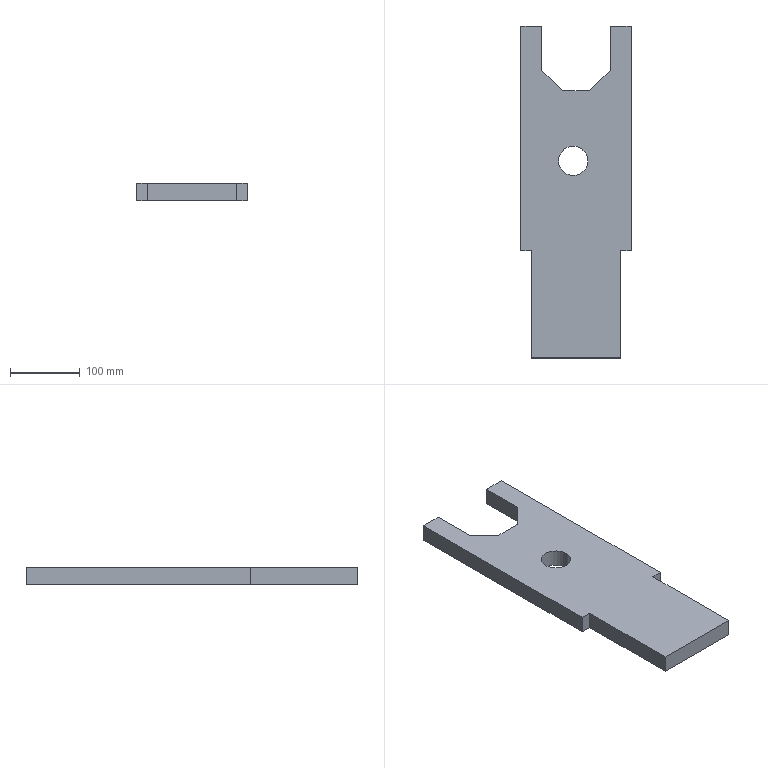Part | STEP file | 03-Plate 1 | 1 solid | 18 faces | box 158 x 475 x 25 mm | volume 1521139 mm3 | plane 16 | cylinder 2 | commonest cylinder face diameters 42 x2
STEP:
#1=CARTESIAN_POINT('',(0.,0.,0.));
#2=DIRECTION('',(0.,0.,1.));
#3=DIRECTION('',(1.,0.,0.));
#4=AXIS2_PLACEMENT_3D('',#1,#2,#3);
#5=CARTESIAN_POINT('',(54.,-193.,25.));
#6=VERTEX_POINT('',#5);
#7=CARTESIAN_POINT('',(54.,-193.,0.));
#8=VERTEX_POINT('',#7);
#9=CARTESIAN_POINT('',(54.,-193.,140.));
#10=DIRECTION('',(0.,0.,-1.));
#11=VECTOR('',#10,1.);
#12=LINE('',#9,#11);
#13=CARTESIAN_POINT('',(75.,-193.,140.));
#14=DIRECTION('',(0.,0.,-1.));
#15=DIRECTION('',(-1.,0.,0.));
#16=AXIS2_PLACEMENT_3D('',#13,#14,#15);
#17=CYLINDRICAL_SURFACE('',#16,21.);
#18=CARTESIAN_POINT('',(6.283,0.));
#19=DIRECTION('',(0.,1.));
#20=VECTOR('',#19,1.);
#21=LINE('',#18,#20);
#22=(GEOMETRIC_REPRESENTATION_CONTEXT(2)PARAMETRIC_REPRESENTATION_CONTEXT()REPRESENTATION_CONTEXT('',''));
#23=DEFINITIONAL_REPRESENTATION('',(#21),#22);
#24=PCURVE('',#17,#23);
#25=CARTESIAN_POINT('',(75.,-193.,140.));
#26=DIRECTION('',(0.,0.,-1.));
#27=DIRECTION('',(-1.,0.,0.));
#28=AXIS2_PLACEMENT_3D('',#25,#26,#27);
#29=CYLINDRICAL_SURFACE('',#28,21.);
#30=CARTESIAN_POINT('',(0.,0.));
#31=DIRECTION('',(0.,1.));
#32=VECTOR('',#31,1.);
#33=LINE('',#30,#32);
#34=(GEOMETRIC_REPRESENTATION_CONTEXT(2)PARAMETRIC_REPRESENTATION_CONTEXT()REPRESENTATION_CONTEXT('',''));
#35=DEFINITIONAL_REPRESENTATION('',(#33),#34);
#36=PCURVE('',#29,#35);
#37=SURFACE_CURVE('',#12,(#24,#36),.PCURVE_S1.);
#38=EDGE_CURVE('',#6,#8,#37,.T.);
#39=ORIENTED_EDGE('',*,*,#38,.T.);
#40=CARTESIAN_POINT('',(96.,-193.,0.));
#41=VERTEX_POINT('',#40);
#42=CARTESIAN_POINT('',(75.,-193.,0.));
#43=DIRECTION('',(0.,0.,-1.));
#44=DIRECTION('',(-1.,0.,0.));
#45=AXIS2_PLACEMENT_3D('',#42,#43,#44);
#46=CIRCLE('',#45,21.);
#47=CARTESIAN_POINT('',(0.,140.));
#48=DIRECTION('',(1.,0.));
#49=VECTOR('',#48,1.);
#50=LINE('',#47,#49);
#51=(GEOMETRIC_REPRESENTATION_CONTEXT(2)PARAMETRIC_REPRESENTATION_CONTEXT()REPRESENTATION_CONTEXT('',''));
#52=DEFINITIONAL_REPRESENTATION('',(#50),#51);
#53=PCURVE('',#17,#52);
#54=CARTESIAN_POINT('',(0.,0.,0.));
#55=DIRECTION('',(0.,0.,1.));
#56=DIRECTION('',(1.,0.,0.));
#57=AXIS2_PLACEMENT_3D('',#54,#55,#56);
#58=PLANE('',#57);
#59=CARTESIAN_POINT('',(54.,-193.));
#60=CARTESIAN_POINT('',(54.,-156.627));
#61=CARTESIAN_POINT('',(85.5,-174.813));
#62=CARTESIAN_POINT('',(117.,-193.));
#63=CARTESIAN_POINT('',(85.5,-211.187));
#64=CARTESIAN_POINT('',(54.,-229.373));
#65=CARTESIAN_POINT('',(54.,-193.));
#66=(BOUNDED_CURVE()B_SPLINE_CURVE(2,(#59,#60,#61,#62,#63,#64,#65),.UNSPECIFIED.,.T.,.F.)B_SPLINE_CURVE_WITH_KNOTS((1,2,2,2,2,1),(-2.094,0.,2.094,4.189,6.283,8.378),.UNSPECIFIED.)CURVE()GEOMETRIC_REPRESENTATION_ITEM()RATIONAL_B_SPLINE_CURVE((1.,0.5,1.,0.5,1.,0.5,1.))REPRESENTATION_ITEM(''));
#67=(GEOMETRIC_REPRESENTATION_CONTEXT(2)PARAMETRIC_REPRESENTATION_CONTEXT()REPRESENTATION_CONTEXT('',''));
#68=DEFINITIONAL_REPRESENTATION('',(#66),#67);
#69=PCURVE('',#58,#68);
#70=SURFACE_CURVE('',#46,(#53,#69),.PCURVE_S1.);
#71=EDGE_CURVE('',#41,#8,#70,.T.);
#72=ORIENTED_EDGE('',*,*,#71,.F.);
#73=CARTESIAN_POINT('',(96.,-193.,25.));
#74=VERTEX_POINT('',#73);
#75=CARTESIAN_POINT('',(96.,-193.,140.));
#76=DIRECTION('',(0.,0.,-1.));
#77=VECTOR('',#76,1.);
#78=LINE('',#75,#77);
#79=CARTESIAN_POINT('',(3.142,0.));
#80=DIRECTION('',(0.,1.));
#81=VECTOR('',#80,1.);
#82=LINE('',#79,#81);
#83=(GEOMETRIC_REPRESENTATION_CONTEXT(2)PARAMETRIC_REPRESENTATION_CONTEXT()REPRESENTATION_CONTEXT('',''));
#84=DEFINITIONAL_REPRESENTATION('',(#82),#83);
#85=PCURVE('',#17,#84);
#86=CARTESIAN_POINT('',(3.142,0.));
#87=DIRECTION('',(0.,1.));
#88=VECTOR('',#87,1.);
#89=LINE('',#86,#88);
#90=(GEOMETRIC_REPRESENTATION_CONTEXT(2)PARAMETRIC_REPRESENTATION_CONTEXT()REPRESENTATION_CONTEXT('',''));
#91=DEFINITIONAL_REPRESENTATION('',(#89),#90);
#92=PCURVE('',#29,#91);
#93=SURFACE_CURVE('',#78,(#85,#92),.PCURVE_S1.);
#94=EDGE_CURVE('',#74,#41,#93,.T.);
#95=ORIENTED_EDGE('',*,*,#94,.F.);
#96=CARTESIAN_POINT('',(75.,-193.,25.));
#97=DIRECTION('',(0.,0.,1.));
#98=DIRECTION('',(1.,0.,0.));
#99=AXIS2_PLACEMENT_3D('',#96,#97,#98);
#100=CIRCLE('',#99,21.);
#101=CARTESIAN_POINT('',(9.425,115.));
#102=DIRECTION('',(-1.,0.));
#103=VECTOR('',#102,1.);
#104=LINE('',#101,#103);
#105=(GEOMETRIC_REPRESENTATION_CONTEXT(2)PARAMETRIC_REPRESENTATION_CONTEXT()REPRESENTATION_CONTEXT('',''));
#106=DEFINITIONAL_REPRESENTATION('',(#104),#105);
#107=PCURVE('',#17,#106);
#108=CARTESIAN_POINT('',(0.,0.,25.));
#109=DIRECTION('',(0.,0.,1.));
#110=DIRECTION('',(1.,0.,0.));
#111=AXIS2_PLACEMENT_3D('',#108,#109,#110);
#112=PLANE('',#111);
#113=CARTESIAN_POINT('',(75.,-193.));
#114=DIRECTION('',(1.,0.));
#115=AXIS2_PLACEMENT_2D('',#113,#114);
#116=CIRCLE('',#115,21.);
#117=(GEOMETRIC_REPRESENTATION_CONTEXT(2)PARAMETRIC_REPRESENTATION_CONTEXT()REPRESENTATION_CONTEXT('',''));
#118=DEFINITIONAL_REPRESENTATION('',(#116),#117);
#119=PCURVE('',#112,#118);
#120=SURFACE_CURVE('',#100,(#107,#119),.PCURVE_S1.);
#121=EDGE_CURVE('',#6,#74,#120,.T.);
#122=ORIENTED_EDGE('',*,*,#121,.F.);
#123=EDGE_LOOP('',(#39,#72,#95,#122));
#124=FACE_BOUND('',#123,.F.);
#125=ADVANCED_FACE('',(#124),#17,.F.);
#126=CARTESIAN_POINT('',(0.,0.,0.));
#127=VERTEX_POINT('',#126);
#128=CARTESIAN_POINT('',(0.,-321.5,0.));
#129=VERTEX_POINT('',#128);
#130=CARTESIAN_POINT('',(0.,0.,0.));
#131=DIRECTION('',(0.,-1.,0.));
#132=VECTOR('',#131,1.);
#133=LINE('',#130,#132);
#134=CARTESIAN_POINT('',(0.,0.,25.));
#135=DIRECTION('',(1.,0.,0.));
#136=DIRECTION('',(0.,1.,0.));
#137=AXIS2_PLACEMENT_3D('',#134,#135,#136);
#138=PLANE('',#137);
#139=CARTESIAN_POINT('',(0.,-25.));
#140=DIRECTION('',(-1.,0.));
#141=VECTOR('',#140,1.);
#142=LINE('',#139,#141);
#143=(GEOMETRIC_REPRESENTATION_CONTEXT(2)PARAMETRIC_REPRESENTATION_CONTEXT()REPRESENTATION_CONTEXT('',''));
#144=DEFINITIONAL_REPRESENTATION('',(#142),#143);
#145=PCURVE('',#138,#144);
#146=CARTESIAN_POINT('',(0.,0.));
#147=DIRECTION('',(0.,-1.));
#148=VECTOR('',#147,1.);
#149=LINE('',#146,#148);
#150=(GEOMETRIC_REPRESENTATION_CONTEXT(2)PARAMETRIC_REPRESENTATION_CONTEXT()REPRESENTATION_CONTEXT('',''));
#151=DEFINITIONAL_REPRESENTATION('',(#149),#150);
#152=PCURVE('',#58,#151);
#153=SURFACE_CURVE('',#133,(#145,#152),.PCURVE_S1.);
#154=EDGE_CURVE('',#127,#129,#153,.T.);
#155=ORIENTED_EDGE('',*,*,#154,.T.);
#156=CARTESIAN_POINT('',(0.,-321.5,25.));
#157=VERTEX_POINT('',#156);
#158=CARTESIAN_POINT('',(0.,-321.5,25.));
#159=DIRECTION('',(0.,0.,-1.));
#160=VECTOR('',#159,1.);
#161=LINE('',#158,#160);
#162=CARTESIAN_POINT('',(-321.5,0.));
#163=DIRECTION('',(0.,-1.));
#164=VECTOR('',#163,1.);
#165=LINE('',#162,#164);
#166=(GEOMETRIC_REPRESENTATION_CONTEXT(2)PARAMETRIC_REPRESENTATION_CONTEXT()REPRESENTATION_CONTEXT('',''));
#167=DEFINITIONAL_REPRESENTATION('',(#165),#166);
#168=PCURVE('',#138,#167);
#169=CARTESIAN_POINT('',(0.,-321.5,25.));
#170=DIRECTION('',(0.,1.,0.));
#171=DIRECTION('',(0.,0.,1.));
#172=AXIS2_PLACEMENT_3D('',#169,#170,#171);
#173=PLANE('',#172);
#174=CARTESIAN_POINT('',(0.,0.));
#175=DIRECTION('',(-1.,0.));
#176=VECTOR('',#175,1.);
#177=LINE('',#174,#176);
#178=(GEOMETRIC_REPRESENTATION_CONTEXT(2)PARAMETRIC_REPRESENTATION_CONTEXT()REPRESENTATION_CONTEXT('',''));
#179=DEFINITIONAL_REPRESENTATION('',(#177),#178);
#180=PCURVE('',#173,#179);
#181=SURFACE_CURVE('',#161,(#168,#180),.PCURVE_S1.);
#182=EDGE_CURVE('',#157,#129,#181,.T.);
#183=ORIENTED_EDGE('',*,*,#182,.F.);
#184=CARTESIAN_POINT('',(0.,0.,25.));
#185=VERTEX_POINT('',#184);
#186=CARTESIAN_POINT('',(0.,0.,25.));
#187=DIRECTION('',(0.,-1.,0.));
#188=VECTOR('',#187,1.);
#189=LINE('',#186,#188);
#190=CARTESIAN_POINT('',(0.,0.));
#191=DIRECTION('',(-1.,0.));
#192=VECTOR('',#191,1.);
#193=LINE('',#190,#192);
#194=(GEOMETRIC_REPRESENTATION_CONTEXT(2)PARAMETRIC_REPRESENTATION_CONTEXT()REPRESENTATION_CONTEXT('',''));
#195=DEFINITIONAL_REPRESENTATION('',(#193),#194);
#196=PCURVE('',#138,#195);
#197=CARTESIAN_POINT('',(0.,0.));
#198=DIRECTION('',(0.,-1.));
#199=VECTOR('',#198,1.);
#200=LINE('',#197,#199);
#201=(GEOMETRIC_REPRESENTATION_CONTEXT(2)PARAMETRIC_REPRESENTATION_CONTEXT()REPRESENTATION_CONTEXT('',''));
#202=DEFINITIONAL_REPRESENTATION('',(#200),#201);
#203=PCURVE('',#112,#202);
#204=SURFACE_CURVE('',#189,(#196,#203),.PCURVE_S1.);
#205=EDGE_CURVE('',#185,#157,#204,.T.);
#206=ORIENTED_EDGE('',*,*,#205,.F.);
#207=CARTESIAN_POINT('',(0.,0.,25.));
#208=DIRECTION('',(0.,0.,-1.));
#209=VECTOR('',#208,1.);
#210=LINE('',#207,#209);
#211=CARTESIAN_POINT('',(0.,0.));
#212=DIRECTION('',(0.,-1.));
#213=VECTOR('',#212,1.);
#214=LINE('',#211,#213);
#215=(GEOMETRIC_REPRESENTATION_CONTEXT(2)PARAMETRIC_REPRESENTATION_CONTEXT()REPRESENTATION_CONTEXT('',''));
#216=DEFINITIONAL_REPRESENTATION('',(#214),#215);
#217=PCURVE('',#138,#216);
#218=CARTESIAN_POINT('',(0.,0.,25.));
#219=DIRECTION('',(0.,-1.,0.));
#220=DIRECTION('',(0.,0.,-1.));
#221=AXIS2_PLACEMENT_3D('',#218,#219,#220);
#222=PLANE('',#221);
#223=CARTESIAN_POINT('',(0.,0.));
#224=DIRECTION('',(1.,0.));
#225=VECTOR('',#224,1.);
#226=LINE('',#223,#225);
#227=(GEOMETRIC_REPRESENTATION_CONTEXT(2)PARAMETRIC_REPRESENTATION_CONTEXT()REPRESENTATION_CONTEXT('',''));
#228=DEFINITIONAL_REPRESENTATION('',(#226),#227);
#229=PCURVE('',#222,#228);
#230=SURFACE_CURVE('',#210,(#217,#229),.PCURVE_S1.);
#231=EDGE_CURVE('',#185,#127,#230,.T.);
#232=ORIENTED_EDGE('',*,*,#231,.T.);
#233=EDGE_LOOP('',(#155,#183,#206,#232));
#234=FACE_BOUND('',#233,.T.);
#235=ADVANCED_FACE('',(#234),#138,.F.);
#236=CARTESIAN_POINT('',(15.,-321.5,0.));
#237=VERTEX_POINT('',#236);
#238=CARTESIAN_POINT('',(0.,-321.5,0.));
#239=DIRECTION('',(1.,0.,0.));
#240=VECTOR('',#239,1.);
#241=LINE('',#238,#240);
#242=CARTESIAN_POINT('',(-25.,0.));
#243=DIRECTION('',(0.,1.));
#244=VECTOR('',#243,1.);
#245=LINE('',#242,#244);
#246=(GEOMETRIC_REPRESENTATION_CONTEXT(2)PARAMETRIC_REPRESENTATION_CONTEXT()REPRESENTATION_CONTEXT('',''));
#247=DEFINITIONAL_REPRESENTATION('',(#245),#246);
#248=PCURVE('',#173,#247);
#249=CARTESIAN_POINT('',(0.,-321.5));
#250=DIRECTION('',(1.,0.));
#251=VECTOR('',#250,1.);
#252=LINE('',#249,#251);
#253=(GEOMETRIC_REPRESENTATION_CONTEXT(2)PARAMETRIC_REPRESENTATION_CONTEXT()REPRESENTATION_CONTEXT('',''));
#254=DEFINITIONAL_REPRESENTATION('',(#252),#253);
#255=PCURVE('',#58,#254);
#256=SURFACE_CURVE('',#241,(#248,#255),.PCURVE_S1.);
#257=EDGE_CURVE('',#129,#237,#256,.T.);
#258=ORIENTED_EDGE('',*,*,#257,.T.);
#259=CARTESIAN_POINT('',(15.,-321.5,25.));
#260=VERTEX_POINT('',#259);
#261=CARTESIAN_POINT('',(15.,-321.5,25.));
#262=DIRECTION('',(0.,0.,-1.));
#263=VECTOR('',#262,1.);
#264=LINE('',#261,#263);
#265=CARTESIAN_POINT('',(0.,15.));
#266=DIRECTION('',(-1.,0.));
#267=VECTOR('',#266,1.);
#268=LINE('',#265,#267);
#269=(GEOMETRIC_REPRESENTATION_CONTEXT(2)PARAMETRIC_REPRESENTATION_CONTEXT()REPRESENTATION_CONTEXT('',''));
#270=DEFINITIONAL_REPRESENTATION('',(#268),#269);
#271=PCURVE('',#173,#270);
#272=CARTESIAN_POINT('',(15.,-321.5,25.));
#273=DIRECTION('',(1.,0.,0.));
#274=DIRECTION('',(0.,1.,0.));
#275=AXIS2_PLACEMENT_3D('',#272,#273,#274);
#276=PLANE('',#275);
#277=CARTESIAN_POINT('',(0.,0.));
#278=DIRECTION('',(0.,-1.));
#279=VECTOR('',#278,1.);
#280=LINE('',#277,#279);
#281=(GEOMETRIC_REPRESENTATION_CONTEXT(2)PARAMETRIC_REPRESENTATION_CONTEXT()REPRESENTATION_CONTEXT('',''));
#282=DEFINITIONAL_REPRESENTATION('',(#280),#281);
#283=PCURVE('',#276,#282);
#284=SURFACE_CURVE('',#264,(#271,#283),.PCURVE_S1.);
#285=EDGE_CURVE('',#260,#237,#284,.T.);
#286=ORIENTED_EDGE('',*,*,#285,.F.);
#287=CARTESIAN_POINT('',(0.,-321.5,25.));
#288=DIRECTION('',(1.,0.,0.));
#289=VECTOR('',#288,1.);
#290=LINE('',#287,#289);
#291=CARTESIAN_POINT('',(0.,0.));
#292=DIRECTION('',(0.,1.));
#293=VECTOR('',#292,1.);
#294=LINE('',#291,#293);
#295=(GEOMETRIC_REPRESENTATION_CONTEXT(2)PARAMETRIC_REPRESENTATION_CONTEXT()REPRESENTATION_CONTEXT('',''));
#296=DEFINITIONAL_REPRESENTATION('',(#294),#295);
#297=PCURVE('',#173,#296);
#298=CARTESIAN_POINT('',(0.,-321.5));
#299=DIRECTION('',(1.,0.));
#300=VECTOR('',#299,1.);
#301=LINE('',#298,#300);
#302=(GEOMETRIC_REPRESENTATION_CONTEXT(2)PARAMETRIC_REPRESENTATION_CONTEXT()REPRESENTATION_CONTEXT('',''));
#303=DEFINITIONAL_REPRESENTATION('',(#301),#302);
#304=PCURVE('',#112,#303);
#305=SURFACE_CURVE('',#290,(#297,#304),.PCURVE_S1.);
#306=EDGE_CURVE('',#157,#260,#305,.T.);
#307=ORIENTED_EDGE('',*,*,#306,.F.);
#308=ORIENTED_EDGE('',*,*,#182,.T.);
#309=EDGE_LOOP('',(#258,#286,#307,#308));
#310=FACE_BOUND('',#309,.T.);
#311=ADVANCED_FACE('',(#310),#173,.F.);
#312=CARTESIAN_POINT('',(15.,-475.,0.));
#313=VERTEX_POINT('',#312);
#314=CARTESIAN_POINT('',(15.,-321.5,0.));
#315=DIRECTION('',(0.,-1.,0.));
#316=VECTOR('',#315,1.);
#317=LINE('',#314,#316);
#318=CARTESIAN_POINT('',(0.,-25.));
#319=DIRECTION('',(-1.,0.));
#320=VECTOR('',#319,1.);
#321=LINE('',#318,#320);
#322=(GEOMETRIC_REPRESENTATION_CONTEXT(2)PARAMETRIC_REPRESENTATION_CONTEXT()REPRESENTATION_CONTEXT('',''));
#323=DEFINITIONAL_REPRESENTATION('',(#321),#322);
#324=PCURVE('',#276,#323);
#325=CARTESIAN_POINT('',(15.,-321.5));
#326=DIRECTION('',(0.,-1.));
#327=VECTOR('',#326,1.);
#328=LINE('',#325,#327);
#329=(GEOMETRIC_REPRESENTATION_CONTEXT(2)PARAMETRIC_REPRESENTATION_CONTEXT()REPRESENTATION_CONTEXT('',''));
#330=DEFINITIONAL_REPRESENTATION('',(#328),#329);
#331=PCURVE('',#58,#330);
#332=SURFACE_CURVE('',#317,(#324,#331),.PCURVE_S1.);
#333=EDGE_CURVE('',#237,#313,#332,.T.);
#334=ORIENTED_EDGE('',*,*,#333,.T.);
#335=CARTESIAN_POINT('',(15.,-475.,25.));
#336=VERTEX_POINT('',#335);
#337=CARTESIAN_POINT('',(15.,-475.,25.));
#338=DIRECTION('',(0.,0.,-1.));
#339=VECTOR('',#338,1.);
#340=LINE('',#337,#339);
#341=CARTESIAN_POINT('',(-153.5,0.));
#342=DIRECTION('',(0.,-1.));
#343=VECTOR('',#342,1.);
#344=LINE('',#341,#343);
#345=(GEOMETRIC_REPRESENTATION_CONTEXT(2)PARAMETRIC_REPRESENTATION_CONTEXT()REPRESENTATION_CONTEXT('',''));
#346=DEFINITIONAL_REPRESENTATION('',(#344),#345);
#347=PCURVE('',#276,#346);
#348=CARTESIAN_POINT('',(15.,-475.,25.));
#349=DIRECTION('',(0.,1.,0.));
#350=DIRECTION('',(-1.,0.,0.));
#351=AXIS2_PLACEMENT_3D('',#348,#349,#350);
#352=PLANE('',#351);
#353=CARTESIAN_POINT('',(0.,0.));
#354=DIRECTION('',(0.,-1.));
#355=VECTOR('',#354,1.);
#356=LINE('',#353,#355);
#357=(GEOMETRIC_REPRESENTATION_CONTEXT(2)PARAMETRIC_REPRESENTATION_CONTEXT()REPRESENTATION_CONTEXT('',''));
#358=DEFINITIONAL_REPRESENTATION('',(#356),#357);
#359=PCURVE('',#352,#358);
#360=SURFACE_CURVE('',#340,(#347,#359),.PCURVE_S1.);
#361=EDGE_CURVE('',#336,#313,#360,.T.);
#362=ORIENTED_EDGE('',*,*,#361,.F.);
#363=CARTESIAN_POINT('',(15.,-321.5,25.));
#364=DIRECTION('',(0.,-1.,0.));
#365=VECTOR('',#364,1.);
#366=LINE('',#363,#365);
#367=CARTESIAN_POINT('',(0.,0.));
#368=DIRECTION('',(-1.,0.));
#369=VECTOR('',#368,1.);
#370=LINE('',#367,#369);
#371=(GEOMETRIC_REPRESENTATION_CONTEXT(2)PARAMETRIC_REPRESENTATION_CONTEXT()REPRESENTATION_CONTEXT('',''));
#372=DEFINITIONAL_REPRESENTATION('',(#370),#371);
#373=PCURVE('',#276,#372);
#374=CARTESIAN_POINT('',(15.,-321.5));
#375=DIRECTION('',(0.,-1.));
#376=VECTOR('',#375,1.);
#377=LINE('',#374,#376);
#378=(GEOMETRIC_REPRESENTATION_CONTEXT(2)PARAMETRIC_REPRESENTATION_CONTEXT()REPRESENTATION_CONTEXT('',''));
#379=DEFINITIONAL_REPRESENTATION('',(#377),#378);
#380=PCURVE('',#112,#379);
#381=SURFACE_CURVE('',#366,(#373,#380),.PCURVE_S1.);
#382=EDGE_CURVE('',#260,#336,#381,.T.);
#383=ORIENTED_EDGE('',*,*,#382,.F.);
#384=ORIENTED_EDGE('',*,*,#285,.T.);
#385=EDGE_LOOP('',(#334,#362,#383,#384));
#386=FACE_BOUND('',#385,.T.);
#387=ADVANCED_FACE('',(#386),#276,.F.);
#388=CARTESIAN_POINT('',(143.,-475.,0.));
#389=VERTEX_POINT('',#388);
#390=CARTESIAN_POINT('',(15.,-475.,0.));
#391=DIRECTION('',(1.,0.,0.));
#392=VECTOR('',#391,1.);
#393=LINE('',#390,#392);
#394=CARTESIAN_POINT('',(0.,-25.));
#395=DIRECTION('',(-1.,0.));
#396=VECTOR('',#395,1.);
#397=LINE('',#394,#396);
#398=(GEOMETRIC_REPRESENTATION_CONTEXT(2)PARAMETRIC_REPRESENTATION_CONTEXT()REPRESENTATION_CONTEXT('',''));
#399=DEFINITIONAL_REPRESENTATION('',(#397),#398);
#400=PCURVE('',#352,#399);
#401=CARTESIAN_POINT('',(15.,-475.));
#402=DIRECTION('',(1.,0.));
#403=VECTOR('',#402,1.);
#404=LINE('',#401,#403);
#405=(GEOMETRIC_REPRESENTATION_CONTEXT(2)PARAMETRIC_REPRESENTATION_CONTEXT()REPRESENTATION_CONTEXT('',''));
#406=DEFINITIONAL_REPRESENTATION('',(#404),#405);
#407=PCURVE('',#58,#406);
#408=SURFACE_CURVE('',#393,(#400,#407),.PCURVE_S1.);
#409=EDGE_CURVE('',#313,#389,#408,.T.);
#410=ORIENTED_EDGE('',*,*,#409,.T.);
#411=CARTESIAN_POINT('',(143.,-475.,25.));
#412=VERTEX_POINT('',#411);
#413=CARTESIAN_POINT('',(143.,-475.,25.));
#414=DIRECTION('',(0.,0.,-1.));
#415=VECTOR('',#414,1.);
#416=LINE('',#413,#415);
#417=CARTESIAN_POINT('',(-128.,0.));
#418=DIRECTION('',(0.,-1.));
#419=VECTOR('',#418,1.);
#420=LINE('',#417,#419);
#421=(GEOMETRIC_REPRESENTATION_CONTEXT(2)PARAMETRIC_REPRESENTATION_CONTEXT()REPRESENTATION_CONTEXT('',''));
#422=DEFINITIONAL_REPRESENTATION('',(#420),#421);
#423=PCURVE('',#352,#422);
#424=CARTESIAN_POINT('',(143.,-321.5,25.));
#425=DIRECTION('',(-1.,0.,0.));
#426=DIRECTION('',(0.,-1.,0.));
#427=AXIS2_PLACEMENT_3D('',#424,#425,#426);
#428=PLANE('',#427);
#429=CARTESIAN_POINT('',(153.5,0.));
#430=DIRECTION('',(0.,-1.));
#431=VECTOR('',#430,1.);
#432=LINE('',#429,#431);
#433=(GEOMETRIC_REPRESENTATION_CONTEXT(2)PARAMETRIC_REPRESENTATION_CONTEXT()REPRESENTATION_CONTEXT('',''));
#434=DEFINITIONAL_REPRESENTATION('',(#432),#433);
#435=PCURVE('',#428,#434);
#436=SURFACE_CURVE('',#416,(#423,#435),.PCURVE_S1.);
#437=EDGE_CURVE('',#412,#389,#436,.T.);
#438=ORIENTED_EDGE('',*,*,#437,.F.);
#439=CARTESIAN_POINT('',(15.,-475.,25.));
#440=DIRECTION('',(1.,0.,0.));
#441=VECTOR('',#440,1.);
#442=LINE('',#439,#441);
#443=CARTESIAN_POINT('',(0.,0.));
#444=DIRECTION('',(-1.,0.));
#445=VECTOR('',#444,1.);
#446=LINE('',#443,#445);
#447=(GEOMETRIC_REPRESENTATION_CONTEXT(2)PARAMETRIC_REPRESENTATION_CONTEXT()REPRESENTATION_CONTEXT('',''));
#448=DEFINITIONAL_REPRESENTATION('',(#446),#447);
#449=PCURVE('',#352,#448);
#450=CARTESIAN_POINT('',(15.,-475.));
#451=DIRECTION('',(1.,0.));
#452=VECTOR('',#451,1.);
#453=LINE('',#450,#452);
#454=(GEOMETRIC_REPRESENTATION_CONTEXT(2)PARAMETRIC_REPRESENTATION_CONTEXT()REPRESENTATION_CONTEXT('',''));
#455=DEFINITIONAL_REPRESENTATION('',(#453),#454);
#456=PCURVE('',#112,#455);
#457=SURFACE_CURVE('',#442,(#449,#456),.PCURVE_S1.);
#458=EDGE_CURVE('',#336,#412,#457,.T.);
#459=ORIENTED_EDGE('',*,*,#458,.F.);
#460=ORIENTED_EDGE('',*,*,#361,.T.);
#461=EDGE_LOOP('',(#410,#438,#459,#460));
#462=FACE_BOUND('',#461,.T.);
#463=ADVANCED_FACE('',(#462),#352,.F.);
#464=CARTESIAN_POINT('',(143.,-321.5,0.));
#465=VERTEX_POINT('',#464);
#466=CARTESIAN_POINT('',(143.,-321.5,0.));
#467=DIRECTION('',(0.,1.,0.));
#468=VECTOR('',#467,1.);
#469=LINE('',#466,#468);
#470=CARTESIAN_POINT('',(0.,-25.));
#471=DIRECTION('',(-1.,0.));
#472=VECTOR('',#471,1.);
#473=LINE('',#470,#472);
#474=(GEOMETRIC_REPRESENTATION_CONTEXT(2)PARAMETRIC_REPRESENTATION_CONTEXT()REPRESENTATION_CONTEXT('',''));
#475=DEFINITIONAL_REPRESENTATION('',(#473),#474);
#476=PCURVE('',#428,#475);
#477=CARTESIAN_POINT('',(143.,-321.5));
#478=DIRECTION('',(0.,1.));
#479=VECTOR('',#478,1.);
#480=LINE('',#477,#479);
#481=(GEOMETRIC_REPRESENTATION_CONTEXT(2)PARAMETRIC_REPRESENTATION_CONTEXT()REPRESENTATION_CONTEXT('',''));
#482=DEFINITIONAL_REPRESENTATION('',(#480),#481);
#483=PCURVE('',#58,#482);
#484=SURFACE_CURVE('',#469,(#476,#483),.PCURVE_S1.);
#485=EDGE_CURVE('',#389,#465,#484,.T.);
#486=ORIENTED_EDGE('',*,*,#485,.T.);
#487=CARTESIAN_POINT('',(143.,-321.5,25.));
#488=VERTEX_POINT('',#487);
#489=CARTESIAN_POINT('',(143.,-321.5,25.));
#490=DIRECTION('',(0.,0.,-1.));
#491=VECTOR('',#490,1.);
#492=LINE('',#489,#491);
#493=CARTESIAN_POINT('',(0.,0.));
#494=DIRECTION('',(0.,-1.));
#495=VECTOR('',#494,1.);
#496=LINE('',#493,#495);
#497=(GEOMETRIC_REPRESENTATION_CONTEXT(2)PARAMETRIC_REPRESENTATION_CONTEXT()REPRESENTATION_CONTEXT('',''));
#498=DEFINITIONAL_REPRESENTATION('',(#496),#497);
#499=PCURVE('',#428,#498);
#500=CARTESIAN_POINT('',(158.,-321.5,25.));
#501=DIRECTION('',(0.,1.,0.));
#502=DIRECTION('',(0.,0.,1.));
#503=AXIS2_PLACEMENT_3D('',#500,#501,#502);
#504=PLANE('',#503);
#505=CARTESIAN_POINT('',(0.,-15.));
#506=DIRECTION('',(-1.,0.));
#507=VECTOR('',#506,1.);
#508=LINE('',#505,#507);
#509=(GEOMETRIC_REPRESENTATION_CONTEXT(2)PARAMETRIC_REPRESENTATION_CONTEXT()REPRESENTATION_CONTEXT('',''));
#510=DEFINITIONAL_REPRESENTATION('',(#508),#509);
#511=PCURVE('',#504,#510);
#512=SURFACE_CURVE('',#492,(#499,#511),.PCURVE_S1.);
#513=EDGE_CURVE('',#488,#465,#512,.T.);
#514=ORIENTED_EDGE('',*,*,#513,.F.);
#515=CARTESIAN_POINT('',(143.,-321.5,25.));
#516=DIRECTION('',(0.,1.,0.));
#517=VECTOR('',#516,1.);
#518=LINE('',#515,#517);
#519=CARTESIAN_POINT('',(0.,0.));
#520=DIRECTION('',(-1.,0.));
#521=VECTOR('',#520,1.);
#522=LINE('',#519,#521);
#523=(GEOMETRIC_REPRESENTATION_CONTEXT(2)PARAMETRIC_REPRESENTATION_CONTEXT()REPRESENTATION_CONTEXT('',''));
#524=DEFINITIONAL_REPRESENTATION('',(#522),#523);
#525=PCURVE('',#428,#524);
#526=CARTESIAN_POINT('',(143.,-321.5));
#527=DIRECTION('',(0.,1.));
#528=VECTOR('',#527,1.);
#529=LINE('',#526,#528);
#530=(GEOMETRIC_REPRESENTATION_CONTEXT(2)PARAMETRIC_REPRESENTATION_CONTEXT()REPRESENTATION_CONTEXT('',''));
#531=DEFINITIONAL_REPRESENTATION('',(#529),#530);
#532=PCURVE('',#112,#531);
#533=SURFACE_CURVE('',#518,(#525,#532),.PCURVE_S1.);
#534=EDGE_CURVE('',#412,#488,#533,.T.);
#535=ORIENTED_EDGE('',*,*,#534,.F.);
#536=ORIENTED_EDGE('',*,*,#437,.T.);
#537=EDGE_LOOP('',(#486,#514,#535,#536));
#538=FACE_BOUND('',#537,.T.);
#539=ADVANCED_FACE('',(#538),#428,.F.);
#540=CARTESIAN_POINT('',(158.,-321.5,0.));
#541=VERTEX_POINT('',#540);
#542=CARTESIAN_POINT('',(158.,-321.5,0.));
#543=DIRECTION('',(1.,0.,0.));
#544=VECTOR('',#543,1.);
#545=LINE('',#542,#544);
#546=CARTESIAN_POINT('',(-25.,0.));
#547=DIRECTION('',(0.,1.));
#548=VECTOR('',#547,1.);
#549=LINE('',#546,#548);
#550=(GEOMETRIC_REPRESENTATION_CONTEXT(2)PARAMETRIC_REPRESENTATION_CONTEXT()REPRESENTATION_CONTEXT('',''));
#551=DEFINITIONAL_REPRESENTATION('',(#549),#550);
#552=PCURVE('',#504,#551);
#553=CARTESIAN_POINT('',(158.,-321.5));
#554=DIRECTION('',(1.,0.));
#555=VECTOR('',#554,1.);
#556=LINE('',#553,#555);
#557=(GEOMETRIC_REPRESENTATION_CONTEXT(2)PARAMETRIC_REPRESENTATION_CONTEXT()REPRESENTATION_CONTEXT('',''));
#558=DEFINITIONAL_REPRESENTATION('',(#556),#557);
#559=PCURVE('',#58,#558);
#560=SURFACE_CURVE('',#545,(#552,#559),.PCURVE_S1.);
#561=EDGE_CURVE('',#465,#541,#560,.T.);
#562=ORIENTED_EDGE('',*,*,#561,.T.);
#563=CARTESIAN_POINT('',(158.,-321.5,25.));
#564=VERTEX_POINT('',#563);
#565=CARTESIAN_POINT('',(158.,-321.5,25.));
#566=DIRECTION('',(0.,0.,-1.));
#567=VECTOR('',#566,1.);
#568=LINE('',#565,#567);
#569=CARTESIAN_POINT('',(0.,0.));
#570=DIRECTION('',(-1.,0.));
#571=VECTOR('',#570,1.);
#572=LINE('',#569,#571);
#573=(GEOMETRIC_REPRESENTATION_CONTEXT(2)PARAMETRIC_REPRESENTATION_CONTEXT()REPRESENTATION_CONTEXT('',''));
#574=DEFINITIONAL_REPRESENTATION('',(#572),#573);
#575=PCURVE('',#504,#574);
#576=CARTESIAN_POINT('',(158.,0.,25.));
#577=DIRECTION('',(-1.,0.,0.));
#578=DIRECTION('',(0.,0.,1.));
#579=AXIS2_PLACEMENT_3D('',#576,#577,#578);
#580=PLANE('',#579);
#581=CARTESIAN_POINT('',(0.,-321.5));
#582=DIRECTION('',(-1.,0.));
#583=VECTOR('',#582,1.);
#584=LINE('',#581,#583);
#585=(GEOMETRIC_REPRESENTATION_CONTEXT(2)PARAMETRIC_REPRESENTATION_CONTEXT()REPRESENTATION_CONTEXT('',''));
#586=DEFINITIONAL_REPRESENTATION('',(#584),#585);
#587=PCURVE('',#580,#586);
#588=SURFACE_CURVE('',#568,(#575,#587),.PCURVE_S1.);
#589=EDGE_CURVE('',#564,#541,#588,.T.);
#590=ORIENTED_EDGE('',*,*,#589,.F.);
#591=CARTESIAN_POINT('',(158.,-321.5,25.));
#592=DIRECTION('',(1.,0.,0.));
#593=VECTOR('',#592,1.);
#594=LINE('',#591,#593);
#595=CARTESIAN_POINT('',(0.,0.));
#596=DIRECTION('',(0.,1.));
#597=VECTOR('',#596,1.);
#598=LINE('',#595,#597);
#599=(GEOMETRIC_REPRESENTATION_CONTEXT(2)PARAMETRIC_REPRESENTATION_CONTEXT()REPRESENTATION_CONTEXT('',''));
#600=DEFINITIONAL_REPRESENTATION('',(#598),#599);
#601=PCURVE('',#504,#600);
#602=CARTESIAN_POINT('',(158.,-321.5));
#603=DIRECTION('',(1.,0.));
#604=VECTOR('',#603,1.);
#605=LINE('',#602,#604);
#606=(GEOMETRIC_REPRESENTATION_CONTEXT(2)PARAMETRIC_REPRESENTATION_CONTEXT()REPRESENTATION_CONTEXT('',''));
#607=DEFINITIONAL_REPRESENTATION('',(#605),#606);
#608=PCURVE('',#112,#607);
#609=SURFACE_CURVE('',#594,(#601,#608),.PCURVE_S1.);
#610=EDGE_CURVE('',#488,#564,#609,.T.);
#611=ORIENTED_EDGE('',*,*,#610,.F.);
#612=ORIENTED_EDGE('',*,*,#513,.T.);
#613=EDGE_LOOP('',(#562,#590,#611,#612));
#614=FACE_BOUND('',#613,.T.);
#615=ADVANCED_FACE('',(#614),#504,.F.);
#616=CARTESIAN_POINT('',(158.,0.,0.));
#617=VERTEX_POINT('',#616);
#618=CARTESIAN_POINT('',(158.,0.,0.));
#619=DIRECTION('',(0.,1.,0.));
#620=VECTOR('',#619,1.);
#621=LINE('',#618,#620);
#622=CARTESIAN_POINT('',(-25.,0.));
#623=DIRECTION('',(0.,1.));
#624=VECTOR('',#623,1.);
#625=LINE('',#622,#624);
#626=(GEOMETRIC_REPRESENTATION_CONTEXT(2)PARAMETRIC_REPRESENTATION_CONTEXT()REPRESENTATION_CONTEXT('',''));
#627=DEFINITIONAL_REPRESENTATION('',(#625),#626);
#628=PCURVE('',#580,#627);
#629=CARTESIAN_POINT('',(158.,0.));
#630=DIRECTION('',(0.,1.));
#631=VECTOR('',#630,1.);
#632=LINE('',#629,#631);
#633=(GEOMETRIC_REPRESENTATION_CONTEXT(2)PARAMETRIC_REPRESENTATION_CONTEXT()REPRESENTATION_CONTEXT('',''));
#634=DEFINITIONAL_REPRESENTATION('',(#632),#633);
#635=PCURVE('',#58,#634);
#636=SURFACE_CURVE('',#621,(#628,#635),.PCURVE_S1.);
#637=EDGE_CURVE('',#541,#617,#636,.T.);
#638=ORIENTED_EDGE('',*,*,#637,.T.);
#639=CARTESIAN_POINT('',(158.,0.,25.));
#640=VERTEX_POINT('',#639);
#641=CARTESIAN_POINT('',(158.,0.,25.));
#642=DIRECTION('',(0.,0.,-1.));
#643=VECTOR('',#642,1.);
#644=LINE('',#641,#643);
#645=CARTESIAN_POINT('',(0.,0.));
#646=DIRECTION('',(-1.,0.));
#647=VECTOR('',#646,1.);
#648=LINE('',#645,#647);
#649=(GEOMETRIC_REPRESENTATION_CONTEXT(2)PARAMETRIC_REPRESENTATION_CONTEXT()REPRESENTATION_CONTEXT('',''));
#650=DEFINITIONAL_REPRESENTATION('',(#648),#649);
#651=PCURVE('',#580,#650);
#652=CARTESIAN_POINT('',(128.,0.,25.));
#653=DIRECTION('',(0.,-1.,0.));
#654=DIRECTION('',(0.,0.,-1.));
#655=AXIS2_PLACEMENT_3D('',#652,#653,#654);
#656=PLANE('',#655);
#657=CARTESIAN_POINT('',(0.,30.));
#658=DIRECTION('',(1.,0.));
#659=VECTOR('',#658,1.);
#660=LINE('',#657,#659);
#661=(GEOMETRIC_REPRESENTATION_CONTEXT(2)PARAMETRIC_REPRESENTATION_CONTEXT()REPRESENTATION_CONTEXT('',''));
#662=DEFINITIONAL_REPRESENTATION('',(#660),#661);
#663=PCURVE('',#656,#662);
#664=SURFACE_CURVE('',#644,(#651,#663),.PCURVE_S1.);
#665=EDGE_CURVE('',#640,#617,#664,.T.);
#666=ORIENTED_EDGE('',*,*,#665,.F.);
#667=CARTESIAN_POINT('',(158.,0.,25.));
#668=DIRECTION('',(0.,1.,0.));
#669=VECTOR('',#668,1.);
#670=LINE('',#667,#669);
#671=CARTESIAN_POINT('',(0.,0.));
#672=DIRECTION('',(0.,1.));
#673=VECTOR('',#672,1.);
#674=LINE('',#671,#673);
#675=(GEOMETRIC_REPRESENTATION_CONTEXT(2)PARAMETRIC_REPRESENTATION_CONTEXT()REPRESENTATION_CONTEXT('',''));
#676=DEFINITIONAL_REPRESENTATION('',(#674),#675);
#677=PCURVE('',#580,#676);
#678=CARTESIAN_POINT('',(158.,0.));
#679=DIRECTION('',(0.,1.));
#680=VECTOR('',#679,1.);
#681=LINE('',#678,#680);
#682=(GEOMETRIC_REPRESENTATION_CONTEXT(2)PARAMETRIC_REPRESENTATION_CONTEXT()REPRESENTATION_CONTEXT('',''));
#683=DEFINITIONAL_REPRESENTATION('',(#681),#682);
#684=PCURVE('',#112,#683);
#685=SURFACE_CURVE('',#670,(#677,#684),.PCURVE_S1.);
#686=EDGE_CURVE('',#564,#640,#685,.T.);
#687=ORIENTED_EDGE('',*,*,#686,.F.);
#688=ORIENTED_EDGE('',*,*,#589,.T.);
#689=EDGE_LOOP('',(#638,#666,#687,#688));
#690=FACE_BOUND('',#689,.T.);
#691=ADVANCED_FACE('',(#690),#580,.F.);
#692=CARTESIAN_POINT('',(128.,0.,0.));
#693=VERTEX_POINT('',#692);
#694=CARTESIAN_POINT('',(128.,0.,0.));
#695=DIRECTION('',(-1.,0.,0.));
#696=VECTOR('',#695,1.);
#697=LINE('',#694,#696);
#698=CARTESIAN_POINT('',(25.,0.));
#699=DIRECTION('',(0.,-1.));
#700=VECTOR('',#699,1.);
#701=LINE('',#698,#700);
#702=(GEOMETRIC_REPRESENTATION_CONTEXT(2)PARAMETRIC_REPRESENTATION_CONTEXT()REPRESENTATION_CONTEXT('',''));
#703=DEFINITIONAL_REPRESENTATION('',(#701),#702);
#704=PCURVE('',#656,#703);
#705=CARTESIAN_POINT('',(128.,0.));
#706=DIRECTION('',(-1.,0.));
#707=VECTOR('',#706,1.);
#708=LINE('',#705,#707);
#709=(GEOMETRIC_REPRESENTATION_CONTEXT(2)PARAMETRIC_REPRESENTATION_CONTEXT()REPRESENTATION_CONTEXT('',''));
#710=DEFINITIONAL_REPRESENTATION('',(#708),#709);
#711=PCURVE('',#58,#710);
#712=SURFACE_CURVE('',#697,(#704,#711),.PCURVE_S1.);
#713=EDGE_CURVE('',#617,#693,#712,.T.);
#714=ORIENTED_EDGE('',*,*,#713,.T.);
#715=CARTESIAN_POINT('',(128.,0.,25.));
#716=VERTEX_POINT('',#715);
#717=CARTESIAN_POINT('',(128.,0.,25.));
#718=DIRECTION('',(0.,0.,-1.));
#719=VECTOR('',#718,1.);
#720=LINE('',#717,#719);
#721=CARTESIAN_POINT('',(0.,0.));
#722=DIRECTION('',(1.,0.));
#723=VECTOR('',#722,1.);
#724=LINE('',#721,#723);
#725=(GEOMETRIC_REPRESENTATION_CONTEXT(2)PARAMETRIC_REPRESENTATION_CONTEXT()REPRESENTATION_CONTEXT('',''));
#726=DEFINITIONAL_REPRESENTATION('',(#724),#725);
#727=PCURVE('',#656,#726);
#728=CARTESIAN_POINT('',(128.,0.,25.));
#729=DIRECTION('',(1.,0.,0.));
#730=DIRECTION('',(0.,0.,-1.));
#731=AXIS2_PLACEMENT_3D('',#728,#729,#730);
#732=PLANE('',#731);
#733=CARTESIAN_POINT('',(0.,0.));
#734=DIRECTION('',(1.,0.));
#735=VECTOR('',#734,1.);
#736=LINE('',#733,#735);
#737=(GEOMETRIC_REPRESENTATION_CONTEXT(2)PARAMETRIC_REPRESENTATION_CONTEXT()REPRESENTATION_CONTEXT('',''));
#738=DEFINITIONAL_REPRESENTATION('',(#736),#737);
#739=PCURVE('',#732,#738);
#740=SURFACE_CURVE('',#720,(#727,#739),.PCURVE_S1.);
#741=EDGE_CURVE('',#716,#693,#740,.T.);
#742=ORIENTED_EDGE('',*,*,#741,.F.);
#743=CARTESIAN_POINT('',(128.,0.,25.));
#744=DIRECTION('',(-1.,0.,0.));
#745=VECTOR('',#744,1.);
#746=LINE('',#743,#745);
#747=CARTESIAN_POINT('',(0.,0.));
#748=DIRECTION('',(0.,-1.));
#749=VECTOR('',#748,1.);
#750=LINE('',#747,#749);
#751=(GEOMETRIC_REPRESENTATION_CONTEXT(2)PARAMETRIC_REPRESENTATION_CONTEXT()REPRESENTATION_CONTEXT('',''));
#752=DEFINITIONAL_REPRESENTATION('',(#750),#751);
#753=PCURVE('',#656,#752);
#754=CARTESIAN_POINT('',(128.,0.));
#755=DIRECTION('',(-1.,0.));
#756=VECTOR('',#755,1.);
#757=LINE('',#754,#756);
#758=(GEOMETRIC_REPRESENTATION_CONTEXT(2)PARAMETRIC_REPRESENTATION_CONTEXT()REPRESENTATION_CONTEXT('',''));
#759=DEFINITIONAL_REPRESENTATION('',(#757),#758);
#760=PCURVE('',#112,#759);
#761=SURFACE_CURVE('',#746,(#753,#760),.PCURVE_S1.);
#762=EDGE_CURVE('',#640,#716,#761,.T.);
#763=ORIENTED_EDGE('',*,*,#762,.F.);
#764=ORIENTED_EDGE('',*,*,#665,.T.);
#765=EDGE_LOOP('',(#714,#742,#763,#764));
#766=FACE_BOUND('',#765,.T.);
#767=ADVANCED_FACE('',(#766),#656,.F.);
#768=CARTESIAN_POINT('',(128.,-63.,0.));
#769=VERTEX_POINT('',#768);
#770=CARTESIAN_POINT('',(128.,0.,0.));
#771=DIRECTION('',(0.,-1.,0.));
#772=VECTOR('',#771,1.);
#773=LINE('',#770,#772);
#774=CARTESIAN_POINT('',(25.,0.));
#775=DIRECTION('',(0.,-1.));
#776=VECTOR('',#775,1.);
#777=LINE('',#774,#776);
#778=(GEOMETRIC_REPRESENTATION_CONTEXT(2)PARAMETRIC_REPRESENTATION_CONTEXT()REPRESENTATION_CONTEXT('',''));
#779=DEFINITIONAL_REPRESENTATION('',(#777),#778);
#780=PCURVE('',#732,#779);
#781=CARTESIAN_POINT('',(128.,0.));
#782=DIRECTION('',(0.,-1.));
#783=VECTOR('',#782,1.);
#784=LINE('',#781,#783);
#785=(GEOMETRIC_REPRESENTATION_CONTEXT(2)PARAMETRIC_REPRESENTATION_CONTEXT()REPRESENTATION_CONTEXT('',''));
#786=DEFINITIONAL_REPRESENTATION('',(#784),#785);
#787=PCURVE('',#58,#786);
#788=SURFACE_CURVE('',#773,(#780,#787),.PCURVE_S1.);
#789=EDGE_CURVE('',#693,#769,#788,.T.);
#790=ORIENTED_EDGE('',*,*,#789,.T.);
#791=CARTESIAN_POINT('',(128.,-63.,25.));
#792=VERTEX_POINT('',#791);
#793=CARTESIAN_POINT('',(128.,-63.,25.));
#794=DIRECTION('',(0.,0.,-1.));
#795=VECTOR('',#794,1.);
#796=LINE('',#793,#795);
#797=CARTESIAN_POINT('',(0.,-63.));
#798=DIRECTION('',(1.,0.));
#799=VECTOR('',#798,1.);
#800=LINE('',#797,#799);
#801=(GEOMETRIC_REPRESENTATION_CONTEXT(2)PARAMETRIC_REPRESENTATION_CONTEXT()REPRESENTATION_CONTEXT('',''));
#802=DEFINITIONAL_REPRESENTATION('',(#800),#801);
#803=PCURVE('',#732,#802);
#804=CARTESIAN_POINT('',(128.,-63.,25.));
#805=DIRECTION('',(0.7071,-0.7071,0.));
#806=DIRECTION('',(0.7071,0.7071,0.));
#807=AXIS2_PLACEMENT_3D('',#804,#805,#806);
#808=PLANE('',#807);
#809=CARTESIAN_POINT('',(0.,0.));
#810=DIRECTION('',(0.,-1.));
#811=VECTOR('',#810,1.);
#812=LINE('',#809,#811);
#813=(GEOMETRIC_REPRESENTATION_CONTEXT(2)PARAMETRIC_REPRESENTATION_CONTEXT()REPRESENTATION_CONTEXT('',''));
#814=DEFINITIONAL_REPRESENTATION('',(#812),#813);
#815=PCURVE('',#808,#814);
#816=SURFACE_CURVE('',#796,(#803,#815),.PCURVE_S1.);
#817=EDGE_CURVE('',#792,#769,#816,.T.);
#818=ORIENTED_EDGE('',*,*,#817,.F.);
#819=CARTESIAN_POINT('',(128.,0.,25.));
#820=DIRECTION('',(0.,-1.,0.));
#821=VECTOR('',#820,1.);
#822=LINE('',#819,#821);
#823=CARTESIAN_POINT('',(0.,0.));
#824=DIRECTION('',(0.,-1.));
#825=VECTOR('',#824,1.);
#826=LINE('',#823,#825);
#827=(GEOMETRIC_REPRESENTATION_CONTEXT(2)PARAMETRIC_REPRESENTATION_CONTEXT()REPRESENTATION_CONTEXT('',''));
#828=DEFINITIONAL_REPRESENTATION('',(#826),#827);
#829=PCURVE('',#732,#828);
#830=CARTESIAN_POINT('',(128.,0.));
#831=DIRECTION('',(0.,-1.));
#832=VECTOR('',#831,1.);
#833=LINE('',#830,#832);
#834=(GEOMETRIC_REPRESENTATION_CONTEXT(2)PARAMETRIC_REPRESENTATION_CONTEXT()REPRESENTATION_CONTEXT('',''));
#835=DEFINITIONAL_REPRESENTATION('',(#833),#834);
#836=PCURVE('',#112,#835);
#837=SURFACE_CURVE('',#822,(#829,#836),.PCURVE_S1.);
#838=EDGE_CURVE('',#716,#792,#837,.T.);
#839=ORIENTED_EDGE('',*,*,#838,.F.);
#840=ORIENTED_EDGE('',*,*,#741,.T.);
#841=EDGE_LOOP('',(#790,#818,#839,#840));
#842=FACE_BOUND('',#841,.T.);
#843=ADVANCED_FACE('',(#842),#732,.F.);
#844=CARTESIAN_POINT('',(98.,-93.,0.));
#845=VERTEX_POINT('',#844);
#846=CARTESIAN_POINT('',(128.,-63.,0.));
#847=DIRECTION('',(-0.7071,-0.7071,0.));
#848=VECTOR('',#847,1.);
#849=LINE('',#846,#848);
#850=CARTESIAN_POINT('',(0.,-25.));
#851=DIRECTION('',(-1.,0.));
#852=VECTOR('',#851,1.);
#853=LINE('',#850,#852);
#854=(GEOMETRIC_REPRESENTATION_CONTEXT(2)PARAMETRIC_REPRESENTATION_CONTEXT()REPRESENTATION_CONTEXT('',''));
#855=DEFINITIONAL_REPRESENTATION('',(#853),#854);
#856=PCURVE('',#808,#855);
#857=CARTESIAN_POINT('',(128.,-63.));
#858=DIRECTION('',(-0.7071,-0.7071));
#859=VECTOR('',#858,1.);
#860=LINE('',#857,#859);
#861=(GEOMETRIC_REPRESENTATION_CONTEXT(2)PARAMETRIC_REPRESENTATION_CONTEXT()REPRESENTATION_CONTEXT('',''));
#862=DEFINITIONAL_REPRESENTATION('',(#860),#861);
#863=PCURVE('',#58,#862);
#864=SURFACE_CURVE('',#849,(#856,#863),.PCURVE_S1.);
#865=EDGE_CURVE('',#769,#845,#864,.T.);
#866=ORIENTED_EDGE('',*,*,#865,.T.);
#867=CARTESIAN_POINT('',(98.,-93.,25.));
#868=VERTEX_POINT('',#867);
#869=CARTESIAN_POINT('',(98.,-93.,25.));
#870=DIRECTION('',(0.,0.,-1.));
#871=VECTOR('',#870,1.);
#872=LINE('',#869,#871);
#873=CARTESIAN_POINT('',(-42.426,0.));
#874=DIRECTION('',(0.,-1.));
#875=VECTOR('',#874,1.);
#876=LINE('',#873,#875);
#877=(GEOMETRIC_REPRESENTATION_CONTEXT(2)PARAMETRIC_REPRESENTATION_CONTEXT()REPRESENTATION_CONTEXT('',''));
#878=DEFINITIONAL_REPRESENTATION('',(#876),#877);
#879=PCURVE('',#808,#878);
#880=CARTESIAN_POINT('',(60.,-93.,25.));
#881=DIRECTION('',(0.,-1.,0.));
#882=DIRECTION('',(0.,0.,-1.));
#883=AXIS2_PLACEMENT_3D('',#880,#881,#882);
#884=PLANE('',#883);
#885=CARTESIAN_POINT('',(0.,38.));
#886=DIRECTION('',(1.,0.));
#887=VECTOR('',#886,1.);
#888=LINE('',#885,#887);
#889=(GEOMETRIC_REPRESENTATION_CONTEXT(2)PARAMETRIC_REPRESENTATION_CONTEXT()REPRESENTATION_CONTEXT('',''));
#890=DEFINITIONAL_REPRESENTATION('',(#888),#889);
#891=PCURVE('',#884,#890);
#892=SURFACE_CURVE('',#872,(#879,#891),.PCURVE_S1.);
#893=EDGE_CURVE('',#868,#845,#892,.T.);
#894=ORIENTED_EDGE('',*,*,#893,.F.);
#895=CARTESIAN_POINT('',(128.,-63.,25.));
#896=DIRECTION('',(-0.7071,-0.7071,0.));
#897=VECTOR('',#896,1.);
#898=LINE('',#895,#897);
#899=CARTESIAN_POINT('',(0.,0.));
#900=DIRECTION('',(-1.,0.));
#901=VECTOR('',#900,1.);
#902=LINE('',#899,#901);
#903=(GEOMETRIC_REPRESENTATION_CONTEXT(2)PARAMETRIC_REPRESENTATION_CONTEXT()REPRESENTATION_CONTEXT('',''));
#904=DEFINITIONAL_REPRESENTATION('',(#902),#903);
#905=PCURVE('',#808,#904);
#906=CARTESIAN_POINT('',(128.,-63.));
#907=DIRECTION('',(-0.7071,-0.7071));
#908=VECTOR('',#907,1.);
#909=LINE('',#906,#908);
#910=(GEOMETRIC_REPRESENTATION_CONTEXT(2)PARAMETRIC_REPRESENTATION_CONTEXT()REPRESENTATION_CONTEXT('',''));
#911=DEFINITIONAL_REPRESENTATION('',(#909),#910);
#912=PCURVE('',#112,#911);
#913=SURFACE_CURVE('',#898,(#905,#912),.PCURVE_S1.);
#914=EDGE_CURVE('',#792,#868,#913,.T.);
#915=ORIENTED_EDGE('',*,*,#914,.F.);
#916=ORIENTED_EDGE('',*,*,#817,.T.);
#917=EDGE_LOOP('',(#866,#894,#915,#916));
#918=FACE_BOUND('',#917,.T.);
#919=ADVANCED_FACE('',(#918),#808,.F.);
#920=CARTESIAN_POINT('',(60.,-93.,0.));
#921=VERTEX_POINT('',#920);
#922=CARTESIAN_POINT('',(60.,-93.,0.));
#923=DIRECTION('',(-1.,0.,0.));
#924=VECTOR('',#923,1.);
#925=LINE('',#922,#924);
#926=CARTESIAN_POINT('',(25.,0.));
#927=DIRECTION('',(0.,-1.));
#928=VECTOR('',#927,1.);
#929=LINE('',#926,#928);
#930=(GEOMETRIC_REPRESENTATION_CONTEXT(2)PARAMETRIC_REPRESENTATION_CONTEXT()REPRESENTATION_CONTEXT('',''));
#931=DEFINITIONAL_REPRESENTATION('',(#929),#930);
#932=PCURVE('',#884,#931);
#933=CARTESIAN_POINT('',(60.,-93.));
#934=DIRECTION('',(-1.,0.));
#935=VECTOR('',#934,1.);
#936=LINE('',#933,#935);
#937=(GEOMETRIC_REPRESENTATION_CONTEXT(2)PARAMETRIC_REPRESENTATION_CONTEXT()REPRESENTATION_CONTEXT('',''));
#938=DEFINITIONAL_REPRESENTATION('',(#936),#937);
#939=PCURVE('',#58,#938);
#940=SURFACE_CURVE('',#925,(#932,#939),.PCURVE_S1.);
#941=EDGE_CURVE('',#845,#921,#940,.T.);
#942=ORIENTED_EDGE('',*,*,#941,.T.);
#943=CARTESIAN_POINT('',(60.,-93.,25.));
#944=VERTEX_POINT('',#943);
#945=CARTESIAN_POINT('',(60.,-93.,25.));
#946=DIRECTION('',(0.,0.,-1.));
#947=VECTOR('',#946,1.);
#948=LINE('',#945,#947);
#949=CARTESIAN_POINT('',(0.,0.));
#950=DIRECTION('',(1.,0.));
#951=VECTOR('',#950,1.);
#952=LINE('',#949,#951);
#953=(GEOMETRIC_REPRESENTATION_CONTEXT(2)PARAMETRIC_REPRESENTATION_CONTEXT()REPRESENTATION_CONTEXT('',''));
#954=DEFINITIONAL_REPRESENTATION('',(#952),#953);
#955=PCURVE('',#884,#954);
#956=CARTESIAN_POINT('',(30.,-63.,25.));
#957=DIRECTION('',(-0.7071,-0.7071,0.));
#958=DIRECTION('',(0.7071,-0.7071,0.));
#959=AXIS2_PLACEMENT_3D('',#956,#957,#958);
#960=PLANE('',#959);
#961=CARTESIAN_POINT('',(42.426,0.));
#962=DIRECTION('',(0.,-1.));
#963=VECTOR('',#962,1.);
#964=LINE('',#961,#963);
#965=(GEOMETRIC_REPRESENTATION_CONTEXT(2)PARAMETRIC_REPRESENTATION_CONTEXT()REPRESENTATION_CONTEXT('',''));
#966=DEFINITIONAL_REPRESENTATION('',(#964),#965);
#967=PCURVE('',#960,#966);
#968=SURFACE_CURVE('',#948,(#955,#967),.PCURVE_S1.);
#969=EDGE_CURVE('',#944,#921,#968,.T.);
#970=ORIENTED_EDGE('',*,*,#969,.F.);
#971=CARTESIAN_POINT('',(60.,-93.,25.));
#972=DIRECTION('',(-1.,0.,0.));
#973=VECTOR('',#972,1.);
#974=LINE('',#971,#973);
#975=CARTESIAN_POINT('',(0.,0.));
#976=DIRECTION('',(0.,-1.));
#977=VECTOR('',#976,1.);
#978=LINE('',#975,#977);
#979=(GEOMETRIC_REPRESENTATION_CONTEXT(2)PARAMETRIC_REPRESENTATION_CONTEXT()REPRESENTATION_CONTEXT('',''));
#980=DEFINITIONAL_REPRESENTATION('',(#978),#979);
#981=PCURVE('',#884,#980);
#982=CARTESIAN_POINT('',(60.,-93.));
#983=DIRECTION('',(-1.,0.));
#984=VECTOR('',#983,1.);
#985=LINE('',#982,#984);
#986=(GEOMETRIC_REPRESENTATION_CONTEXT(2)PARAMETRIC_REPRESENTATION_CONTEXT()REPRESENTATION_CONTEXT('',''));
#987=DEFINITIONAL_REPRESENTATION('',(#985),#986);
#988=PCURVE('',#112,#987);
#989=SURFACE_CURVE('',#974,(#981,#988),.PCURVE_S1.);
#990=EDGE_CURVE('',#868,#944,#989,.T.);
#991=ORIENTED_EDGE('',*,*,#990,.F.);
#992=ORIENTED_EDGE('',*,*,#893,.T.);
#993=EDGE_LOOP('',(#942,#970,#991,#992));
#994=FACE_BOUND('',#993,.T.);
#995=ADVANCED_FACE('',(#994),#884,.F.);
#996=CARTESIAN_POINT('',(30.,-63.,0.));
#997=VERTEX_POINT('',#996);
#998=CARTESIAN_POINT('',(30.,-63.,0.));
#999=DIRECTION('',(-0.7071,0.7071,0.));
#1000=VECTOR('',#999,1.);
#1001=LINE('',#998,#1000);
#1002=CARTESIAN_POINT('',(0.,-25.));
#1003=DIRECTION('',(-1.,0.));
#1004=VECTOR('',#1003,1.);
#1005=LINE('',#1002,#1004);
#1006=(GEOMETRIC_REPRESENTATION_CONTEXT(2)PARAMETRIC_REPRESENTATION_CONTEXT()REPRESENTATION_CONTEXT('',''));
#1007=DEFINITIONAL_REPRESENTATION('',(#1005),#1006);
#1008=PCURVE('',#960,#1007);
#1009=CARTESIAN_POINT('',(30.,-63.));
#1010=DIRECTION('',(-0.7071,0.7071));
#1011=VECTOR('',#1010,1.);
#1012=LINE('',#1009,#1011);
#1013=(GEOMETRIC_REPRESENTATION_CONTEXT(2)PARAMETRIC_REPRESENTATION_CONTEXT()REPRESENTATION_CONTEXT('',''));
#1014=DEFINITIONAL_REPRESENTATION('',(#1012),#1013);
#1015=PCURVE('',#58,#1014);
#1016=SURFACE_CURVE('',#1001,(#1008,#1015),.PCURVE_S1.);
#1017=EDGE_CURVE('',#921,#997,#1016,.T.);
#1018=ORIENTED_EDGE('',*,*,#1017,.T.);
#1019=CARTESIAN_POINT('',(30.,-63.,25.));
#1020=VERTEX_POINT('',#1019);
#1021=CARTESIAN_POINT('',(30.,-63.,25.));
#1022=DIRECTION('',(0.,0.,-1.));
#1023=VECTOR('',#1022,1.);
#1024=LINE('',#1021,#1023);
#1025=CARTESIAN_POINT('',(0.,0.));
#1026=DIRECTION('',(0.,-1.));
#1027=VECTOR('',#1026,1.);
#1028=LINE('',#1025,#1027);
#1029=(GEOMETRIC_REPRESENTATION_CONTEXT(2)PARAMETRIC_REPRESENTATION_CONTEXT()REPRESENTATION_CONTEXT('',''));
#1030=DEFINITIONAL_REPRESENTATION('',(#1028),#1029);
#1031=PCURVE('',#960,#1030);
#1032=CARTESIAN_POINT('',(30.,0.,25.));
#1033=DIRECTION('',(-1.,0.,0.));
#1034=DIRECTION('',(0.,0.,1.));
#1035=AXIS2_PLACEMENT_3D('',#1032,#1033,#1034);
#1036=PLANE('',#1035);
#1037=CARTESIAN_POINT('',(0.,-63.));
#1038=DIRECTION('',(-1.,0.));
#1039=VECTOR('',#1038,1.);
#1040=LINE('',#1037,#1039);
#1041=(GEOMETRIC_REPRESENTATION_CONTEXT(2)PARAMETRIC_REPRESENTATION_CONTEXT()REPRESENTATION_CONTEXT('',''));
#1042=DEFINITIONAL_REPRESENTATION('',(#1040),#1041);
#1043=PCURVE('',#1036,#1042);
#1044=SURFACE_CURVE('',#1024,(#1031,#1043),.PCURVE_S1.);
#1045=EDGE_CURVE('',#1020,#997,#1044,.T.);
#1046=ORIENTED_EDGE('',*,*,#1045,.F.);
#1047=CARTESIAN_POINT('',(30.,-63.,25.));
#1048=DIRECTION('',(-0.7071,0.7071,0.));
#1049=VECTOR('',#1048,1.);
#1050=LINE('',#1047,#1049);
#1051=CARTESIAN_POINT('',(0.,0.));
#1052=DIRECTION('',(-1.,0.));
#1053=VECTOR('',#1052,1.);
#1054=LINE('',#1051,#1053);
#1055=(GEOMETRIC_REPRESENTATION_CONTEXT(2)PARAMETRIC_REPRESENTATION_CONTEXT()REPRESENTATION_CONTEXT('',''));
#1056=DEFINITIONAL_REPRESENTATION('',(#1054),#1055);
#1057=PCURVE('',#960,#1056);
#1058=CARTESIAN_POINT('',(30.,-63.));
#1059=DIRECTION('',(-0.7071,0.7071));
#1060=VECTOR('',#1059,1.);
#1061=LINE('',#1058,#1060);
#1062=(GEOMETRIC_REPRESENTATION_CONTEXT(2)PARAMETRIC_REPRESENTATION_CONTEXT()REPRESENTATION_CONTEXT('',''));
#1063=DEFINITIONAL_REPRESENTATION('',(#1061),#1062);
#1064=PCURVE('',#112,#1063);
#1065=SURFACE_CURVE('',#1050,(#1057,#1064),.PCURVE_S1.);
#1066=EDGE_CURVE('',#944,#1020,#1065,.T.);
#1067=ORIENTED_EDGE('',*,*,#1066,.F.);
#1068=ORIENTED_EDGE('',*,*,#969,.T.);
#1069=EDGE_LOOP('',(#1018,#1046,#1067,#1068));
#1070=FACE_BOUND('',#1069,.T.);
#1071=ADVANCED_FACE('',(#1070),#960,.F.);
#1072=CARTESIAN_POINT('',(30.,0.,0.));
#1073=VERTEX_POINT('',#1072);
#1074=CARTESIAN_POINT('',(30.,0.,0.));
#1075=DIRECTION('',(0.,1.,0.));
#1076=VECTOR('',#1075,1.);
#1077=LINE('',#1074,#1076);
#1078=CARTESIAN_POINT('',(-25.,0.));
#1079=DIRECTION('',(0.,1.));
#1080=VECTOR('',#1079,1.);
#1081=LINE('',#1078,#1080);
#1082=(GEOMETRIC_REPRESENTATION_CONTEXT(2)PARAMETRIC_REPRESENTATION_CONTEXT()REPRESENTATION_CONTEXT('',''));
#1083=DEFINITIONAL_REPRESENTATION('',(#1081),#1082);
#1084=PCURVE('',#1036,#1083);
#1085=CARTESIAN_POINT('',(30.,0.));
#1086=DIRECTION('',(0.,1.));
#1087=VECTOR('',#1086,1.);
#1088=LINE('',#1085,#1087);
#1089=(GEOMETRIC_REPRESENTATION_CONTEXT(2)PARAMETRIC_REPRESENTATION_CONTEXT()REPRESENTATION_CONTEXT('',''));
#1090=DEFINITIONAL_REPRESENTATION('',(#1088),#1089);
#1091=PCURVE('',#58,#1090);
#1092=SURFACE_CURVE('',#1077,(#1084,#1091),.PCURVE_S1.);
#1093=EDGE_CURVE('',#997,#1073,#1092,.T.);
#1094=ORIENTED_EDGE('',*,*,#1093,.T.);
#1095=CARTESIAN_POINT('',(30.,0.,25.));
#1096=VERTEX_POINT('',#1095);
#1097=CARTESIAN_POINT('',(30.,0.,25.));
#1098=DIRECTION('',(0.,0.,-1.));
#1099=VECTOR('',#1098,1.);
#1100=LINE('',#1097,#1099);
#1101=CARTESIAN_POINT('',(0.,0.));
#1102=DIRECTION('',(-1.,0.));
#1103=VECTOR('',#1102,1.);
#1104=LINE('',#1101,#1103);
#1105=(GEOMETRIC_REPRESENTATION_CONTEXT(2)PARAMETRIC_REPRESENTATION_CONTEXT()REPRESENTATION_CONTEXT('',''));
#1106=DEFINITIONAL_REPRESENTATION('',(#1104),#1105);
#1107=PCURVE('',#1036,#1106);
#1108=CARTESIAN_POINT('',(0.,30.));
#1109=DIRECTION('',(1.,0.));
#1110=VECTOR('',#1109,1.);
#1111=LINE('',#1108,#1110);
#1112=(GEOMETRIC_REPRESENTATION_CONTEXT(2)PARAMETRIC_REPRESENTATION_CONTEXT()REPRESENTATION_CONTEXT('',''));
#1113=DEFINITIONAL_REPRESENTATION('',(#1111),#1112);
#1114=PCURVE('',#222,#1113);
#1115=SURFACE_CURVE('',#1100,(#1107,#1114),.PCURVE_S1.);
#1116=EDGE_CURVE('',#1096,#1073,#1115,.T.);
#1117=ORIENTED_EDGE('',*,*,#1116,.F.);
#1118=CARTESIAN_POINT('',(30.,0.,25.));
#1119=DIRECTION('',(0.,1.,0.));
#1120=VECTOR('',#1119,1.);
#1121=LINE('',#1118,#1120);
#1122=CARTESIAN_POINT('',(0.,0.));
#1123=DIRECTION('',(0.,1.));
#1124=VECTOR('',#1123,1.);
#1125=LINE('',#1122,#1124);
#1126=(GEOMETRIC_REPRESENTATION_CONTEXT(2)PARAMETRIC_REPRESENTATION_CONTEXT()REPRESENTATION_CONTEXT('',''));
#1127=DEFINITIONAL_REPRESENTATION('',(#1125),#1126);
#1128=PCURVE('',#1036,#1127);
#1129=CARTESIAN_POINT('',(30.,0.));
#1130=DIRECTION('',(0.,1.));
#1131=VECTOR('',#1130,1.);
#1132=LINE('',#1129,#1131);
#1133=(GEOMETRIC_REPRESENTATION_CONTEXT(2)PARAMETRIC_REPRESENTATION_CONTEXT()REPRESENTATION_CONTEXT('',''));
#1134=DEFINITIONAL_REPRESENTATION('',(#1132),#1133);
#1135=PCURVE('',#112,#1134);
#1136=SURFACE_CURVE('',#1121,(#1128,#1135),.PCURVE_S1.);
#1137=EDGE_CURVE('',#1020,#1096,#1136,.T.);
#1138=ORIENTED_EDGE('',*,*,#1137,.F.);
#1139=ORIENTED_EDGE('',*,*,#1045,.T.);
#1140=EDGE_LOOP('',(#1094,#1117,#1138,#1139));
#1141=FACE_BOUND('',#1140,.T.);
#1142=ADVANCED_FACE('',(#1141),#1036,.F.);
#1143=CARTESIAN_POINT('',(0.,0.,0.));
#1144=DIRECTION('',(-1.,0.,0.));
#1145=VECTOR('',#1144,1.);
#1146=LINE('',#1143,#1145);
#1147=CARTESIAN_POINT('',(25.,0.));
#1148=DIRECTION('',(0.,-1.));
#1149=VECTOR('',#1148,1.);
#1150=LINE('',#1147,#1149);
#1151=(GEOMETRIC_REPRESENTATION_CONTEXT(2)PARAMETRIC_REPRESENTATION_CONTEXT()REPRESENTATION_CONTEXT('',''));
#1152=DEFINITIONAL_REPRESENTATION('',(#1150),#1151);
#1153=PCURVE('',#222,#1152);
#1154=CARTESIAN_POINT('',(0.,0.));
#1155=DIRECTION('',(-1.,0.));
#1156=VECTOR('',#1155,1.);
#1157=LINE('',#1154,#1156);
#1158=(GEOMETRIC_REPRESENTATION_CONTEXT(2)PARAMETRIC_REPRESENTATION_CONTEXT()REPRESENTATION_CONTEXT('',''));
#1159=DEFINITIONAL_REPRESENTATION('',(#1157),#1158);
#1160=PCURVE('',#58,#1159);
#1161=SURFACE_CURVE('',#1146,(#1153,#1160),.PCURVE_S1.);
#1162=EDGE_CURVE('',#1073,#127,#1161,.T.);
#1163=ORIENTED_EDGE('',*,*,#1162,.T.);
#1164=ORIENTED_EDGE('',*,*,#231,.F.);
#1165=CARTESIAN_POINT('',(0.,0.,25.));
#1166=DIRECTION('',(-1.,0.,0.));
#1167=VECTOR('',#1166,1.);
#1168=LINE('',#1165,#1167);
#1169=CARTESIAN_POINT('',(0.,0.));
#1170=DIRECTION('',(0.,-1.));
#1171=VECTOR('',#1170,1.);
#1172=LINE('',#1169,#1171);
#1173=(GEOMETRIC_REPRESENTATION_CONTEXT(2)PARAMETRIC_REPRESENTATION_CONTEXT()REPRESENTATION_CONTEXT('',''));
#1174=DEFINITIONAL_REPRESENTATION('',(#1172),#1173);
#1175=PCURVE('',#222,#1174);
#1176=CARTESIAN_POINT('',(0.,0.));
#1177=DIRECTION('',(-1.,0.));
#1178=VECTOR('',#1177,1.);
#1179=LINE('',#1176,#1178);
#1180=(GEOMETRIC_REPRESENTATION_CONTEXT(2)PARAMETRIC_REPRESENTATION_CONTEXT()REPRESENTATION_CONTEXT('',''));
#1181=DEFINITIONAL_REPRESENTATION('',(#1179),#1180);
#1182=PCURVE('',#112,#1181);
#1183=SURFACE_CURVE('',#1168,(#1175,#1182),.PCURVE_S1.);
#1184=EDGE_CURVE('',#1096,#185,#1183,.T.);
#1185=ORIENTED_EDGE('',*,*,#1184,.F.);
#1186=ORIENTED_EDGE('',*,*,#1116,.T.);
#1187=EDGE_LOOP('',(#1163,#1164,#1185,#1186));
#1188=FACE_BOUND('',#1187,.T.);
#1189=ADVANCED_FACE('',(#1188),#222,.F.);
#1190=ORIENTED_EDGE('',*,*,#121,.F.);
#1191=CARTESIAN_POINT('',(75.,-193.,25.));
#1192=DIRECTION('',(0.,0.,1.));
#1193=DIRECTION('',(1.,0.,0.));
#1194=AXIS2_PLACEMENT_3D('',#1191,#1192,#1193);
#1195=CIRCLE('',#1194,21.);
#1196=CARTESIAN_POINT('',(75.,-193.));
#1197=DIRECTION('',(1.,0.));
#1198=AXIS2_PLACEMENT_2D('',#1196,#1197);
#1199=CIRCLE('',#1198,21.);
#1200=(GEOMETRIC_REPRESENTATION_CONTEXT(2)PARAMETRIC_REPRESENTATION_CONTEXT()REPRESENTATION_CONTEXT('',''));
#1201=DEFINITIONAL_REPRESENTATION('',(#1199),#1200);
#1202=PCURVE('',#112,#1201);
#1203=CARTESIAN_POINT('',(3.142,115.));
#1204=DIRECTION('',(-1.,0.));
#1205=VECTOR('',#1204,1.);
#1206=LINE('',#1203,#1205);
#1207=(GEOMETRIC_REPRESENTATION_CONTEXT(2)PARAMETRIC_REPRESENTATION_CONTEXT()REPRESENTATION_CONTEXT('',''));
#1208=DEFINITIONAL_REPRESENTATION('',(#1206),#1207);
#1209=PCURVE('',#29,#1208);
#1210=SURFACE_CURVE('',#1195,(#1202,#1209),.PCURVE_S1.);
#1211=EDGE_CURVE('',#74,#6,#1210,.T.);
#1212=ORIENTED_EDGE('',*,*,#1211,.F.);
#1213=EDGE_LOOP('',(#1190,#1212));
#1214=FACE_BOUND('',#1213,.T.);
#1215=ORIENTED_EDGE('',*,*,#205,.T.);
#1216=ORIENTED_EDGE('',*,*,#306,.T.);
#1217=ORIENTED_EDGE('',*,*,#382,.T.);
#1218=ORIENTED_EDGE('',*,*,#458,.T.);
#1219=ORIENTED_EDGE('',*,*,#534,.T.);
#1220=ORIENTED_EDGE('',*,*,#610,.T.);
#1221=ORIENTED_EDGE('',*,*,#686,.T.);
#1222=ORIENTED_EDGE('',*,*,#762,.T.);
#1223=ORIENTED_EDGE('',*,*,#838,.T.);
#1224=ORIENTED_EDGE('',*,*,#914,.T.);
#1225=ORIENTED_EDGE('',*,*,#990,.T.);
#1226=ORIENTED_EDGE('',*,*,#1066,.T.);
#1227=ORIENTED_EDGE('',*,*,#1137,.T.);
#1228=ORIENTED_EDGE('',*,*,#1184,.T.);
#1229=EDGE_LOOP('',(#1215,#1216,#1217,#1218,#1219,#1220,#1221,#1222,#1223,#1224,#1225,#1226,#1227,#1228));
#1230=FACE_BOUND('',#1229,.T.);
#1231=ADVANCED_FACE('',(#1214,#1230),#112,.T.);
#1232=CARTESIAN_POINT('',(75.,-193.,0.));
#1233=DIRECTION('',(0.,0.,-1.));
#1234=DIRECTION('',(-1.,0.,0.));
#1235=AXIS2_PLACEMENT_3D('',#1232,#1233,#1234);
#1236=CIRCLE('',#1235,21.);
#1237=CARTESIAN_POINT('',(54.,-193.));
#1238=CARTESIAN_POINT('',(54.,-156.627));
#1239=CARTESIAN_POINT('',(85.5,-174.813));
#1240=CARTESIAN_POINT('',(117.,-193.));
#1241=CARTESIAN_POINT('',(85.5,-211.187));
#1242=CARTESIAN_POINT('',(54.,-229.373));
#1243=CARTESIAN_POINT('',(54.,-193.));
#1244=(BOUNDED_CURVE()B_SPLINE_CURVE(2,(#1237,#1238,#1239,#1240,#1241,#1242,#1243),.UNSPECIFIED.,.T.,.F.)B_SPLINE_CURVE_WITH_KNOTS((1,2,2,2,2,1),(-2.094,0.,2.094,4.189,6.283,8.378),.UNSPECIFIED.)CURVE()GEOMETRIC_REPRESENTATION_ITEM()RATIONAL_B_SPLINE_CURVE((1.,0.5,1.,0.5,1.,0.5,1.))REPRESENTATION_ITEM(''));
#1245=(GEOMETRIC_REPRESENTATION_CONTEXT(2)PARAMETRIC_REPRESENTATION_CONTEXT()REPRESENTATION_CONTEXT('',''));
#1246=DEFINITIONAL_REPRESENTATION('',(#1244),#1245);
#1247=PCURVE('',#58,#1246);
#1248=CARTESIAN_POINT('',(0.,140.));
#1249=DIRECTION('',(1.,0.));
#1250=VECTOR('',#1249,1.);
#1251=LINE('',#1248,#1250);
#1252=(GEOMETRIC_REPRESENTATION_CONTEXT(2)PARAMETRIC_REPRESENTATION_CONTEXT()REPRESENTATION_CONTEXT('',''));
#1253=DEFINITIONAL_REPRESENTATION('',(#1251),#1252);
#1254=PCURVE('',#29,#1253);
#1255=SURFACE_CURVE('',#1236,(#1247,#1254),.PCURVE_S1.);
#1256=EDGE_CURVE('',#8,#41,#1255,.T.);
#1257=ORIENTED_EDGE('',*,*,#1256,.F.);
#1258=ORIENTED_EDGE('',*,*,#71,.F.);
#1259=EDGE_LOOP('',(#1257,#1258));
#1260=FACE_BOUND('',#1259,.T.);
#1261=ORIENTED_EDGE('',*,*,#154,.F.);
#1262=ORIENTED_EDGE('',*,*,#1162,.F.);
#1263=ORIENTED_EDGE('',*,*,#1093,.F.);
#1264=ORIENTED_EDGE('',*,*,#1017,.F.);
#1265=ORIENTED_EDGE('',*,*,#941,.F.);
#1266=ORIENTED_EDGE('',*,*,#865,.F.);
#1267=ORIENTED_EDGE('',*,*,#789,.F.);
#1268=ORIENTED_EDGE('',*,*,#713,.F.);
#1269=ORIENTED_EDGE('',*,*,#637,.F.);
#1270=ORIENTED_EDGE('',*,*,#561,.F.);
#1271=ORIENTED_EDGE('',*,*,#485,.F.);
#1272=ORIENTED_EDGE('',*,*,#409,.F.);
#1273=ORIENTED_EDGE('',*,*,#333,.F.);
#1274=ORIENTED_EDGE('',*,*,#257,.F.);
#1275=EDGE_LOOP('',(#1261,#1262,#1263,#1264,#1265,#1266,#1267,#1268,#1269,#1270,#1271,#1272,#1273,#1274));
#1276=FACE_BOUND('',#1275,.T.);
#1277=ADVANCED_FACE('',(#1260,#1276),#58,.F.);
#1278=ORIENTED_EDGE('',*,*,#1256,.F.);
#1279=ORIENTED_EDGE('',*,*,#38,.F.);
#1280=ORIENTED_EDGE('',*,*,#1211,.F.);
#1281=ORIENTED_EDGE('',*,*,#94,.T.);
#1282=EDGE_LOOP('',(#1278,#1279,#1280,#1281));
#1283=FACE_BOUND('',#1282,.F.);
#1284=ADVANCED_FACE('',(#1283),#29,.F.);
#1285=CLOSED_SHELL('',(#125,#235,#311,#387,#463,#539,#615,#691,#767,#843,#919,#995,#1071,#1142,#1189,#1231,#1277,#1284));
#1286=MANIFOLD_SOLID_BREP('',#1285);
#1287=(LENGTH_UNIT()NAMED_UNIT(*)SI_UNIT(.MILLI.,.METRE.));
#1288=UNCERTAINTY_MEASURE_WITH_UNIT(LENGTH_MEASURE(0.0000001),#1287,'','');
#1289=(NAMED_UNIT(*)PLANE_ANGLE_UNIT()SI_UNIT($,.RADIAN.));
#1290=(NAMED_UNIT(*)SI_UNIT($,.STERADIAN.)SOLID_ANGLE_UNIT());
#1291=(GEOMETRIC_REPRESENTATION_CONTEXT(3)GLOBAL_UNCERTAINTY_ASSIGNED_CONTEXT((#1288))GLOBAL_UNIT_ASSIGNED_CONTEXT((#1287,#1289,#1290))REPRESENTATION_CONTEXT('',''));
#1292=ADVANCED_BREP_SHAPE_REPRESENTATION('',(#4,#1286),#1291);